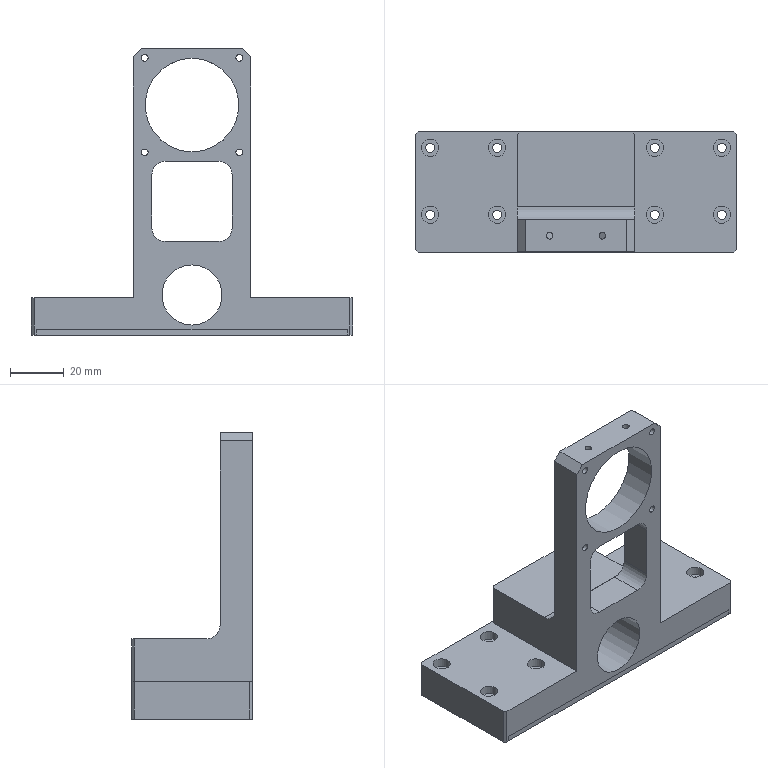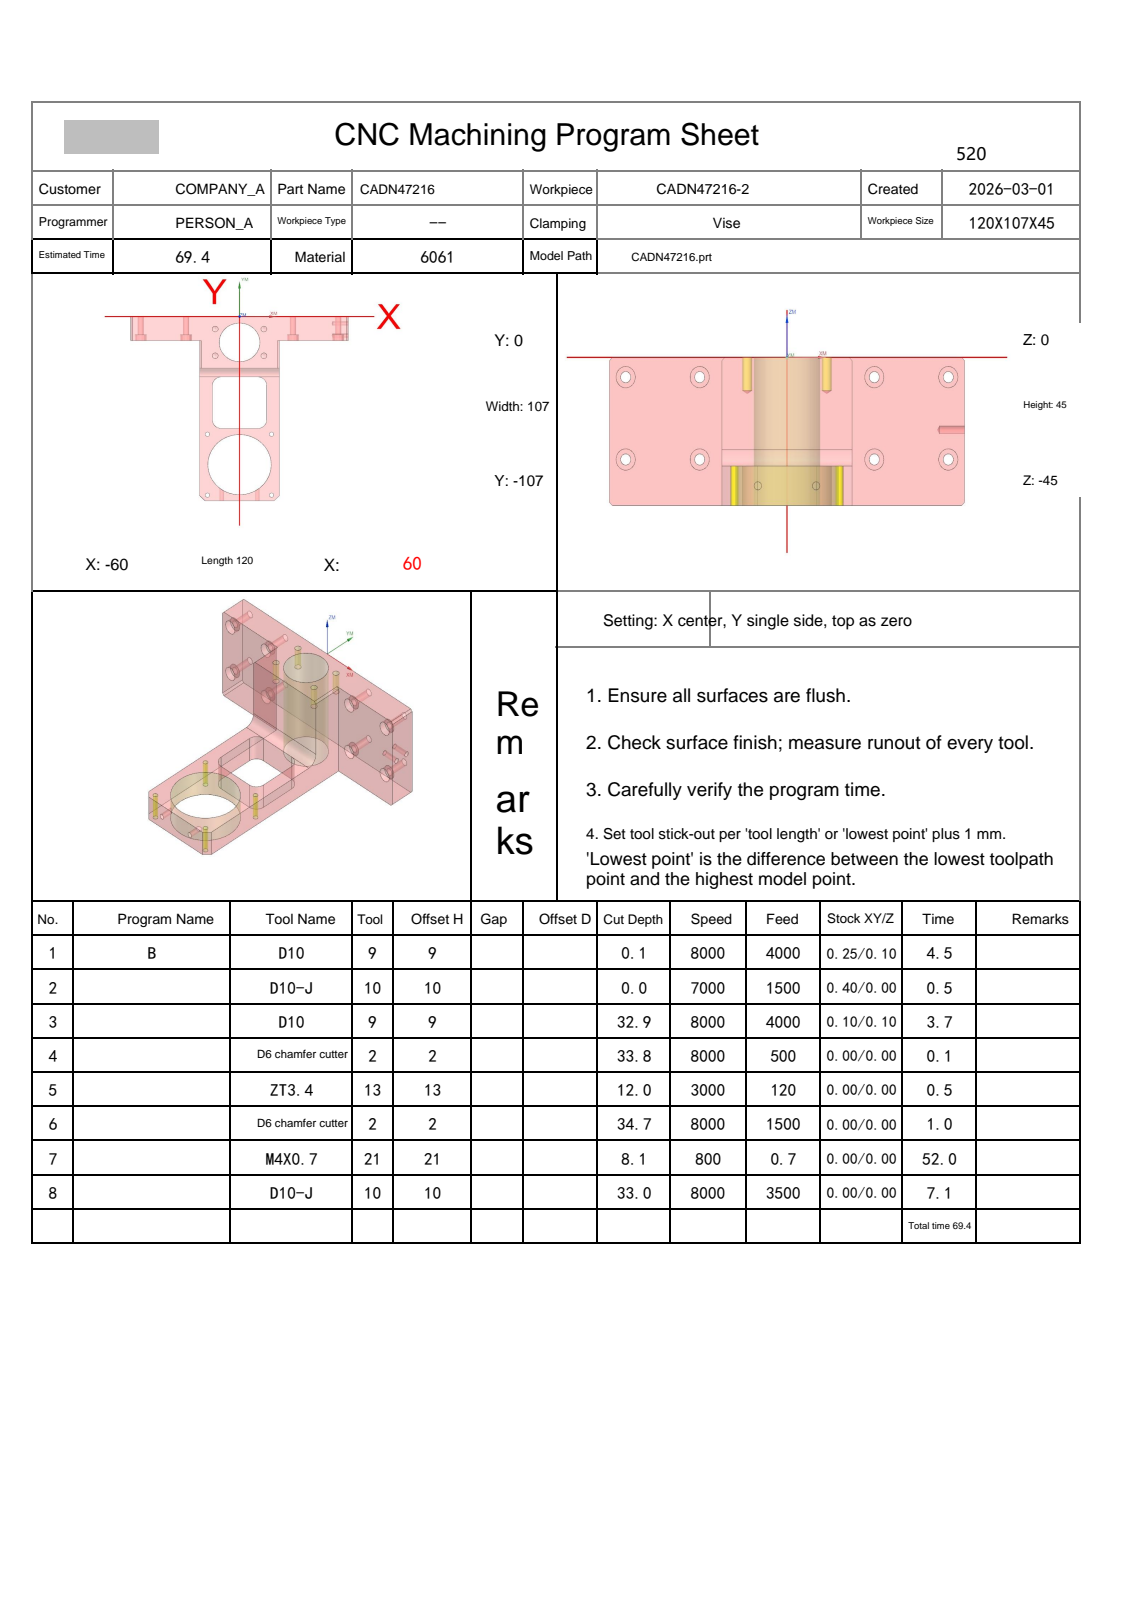NC program | NX | posted by the shop | part box 120 x 45 x 107 mm
Lines 1677 to 1756 of 8568:
N2 T10 M06
(D10-J  D=10. R=0. H=10 ce=0.40 di=0.00)
G00 G90 G54 X-2. Y7. M03 S7000
G43 H10 Z14.5
M08
Z1.5
G01 Z0.0 F1500.
Y3.
G03 X0.0 Y1. I2. J0.0
G01 X59.002
G02 X60. Y.002 I-.002 J-1.
G01 Y-14.002
G02 X59. Y-15. I-1. J.002
G01 X22.
Y-30.002
G02 X21.002 Y-31. I-1. J.002
G01 X-21.002
G02 X-22. Y-30.002 I.002 J1.
G01 Y-15.
X-59.002
G02 X-60. Y-14.002 I.002 J1.
G01 Y.002
G02 X-59.002 Y1. I1. J-.002
G01 X2.086
G02 X2.792 Y.708 I-.001 J-1.
G01 X7.207 Y-3.707
G03 X7.914 Y-4. I.707 J.707
G01 X54.003
G02 X55. Y-4.997 I-.003 J-1.
G01 Y-9.003
G02 X54.003 Y-10. I-1. J.003
G01 X22.
G03 X17. Y-15. I0.0 J-5.
G01 Y-25.003
G02 X16.003 Y-26. I-1. J.003
G01 X-16.003
G02 X-17. Y-25.003 I.003 J1.
G01 Y-15.
G03 X-22. Y-10. I-5. J0.0
G01 X-54.003
G02 X-55. Y-9.003 I.003 J1.
G01 Y-4.997
G02 X-54.003 Y-4. I1. J-.003
G01 X2.086
G02 X2.792 Y-4.292 I-.001 J-1.
G01 X7.207 Y-8.707
G03 X7.914 Y-9. I.707 J.707
G01 X12.205
G02 X13.202 Y-10. I-.003 J-1.
X13.094 Y-10.452 I-1. J0.0
G03 X12. Y-15. I8.906 J-4.548
G01 Y-20.003
G02 X11.003 Y-21. I-1. J.003
G01 X-11.003
G02 X-12. Y-20.003 I.003 J1.
G01 Y-15.
G03 X-13.094 Y-10.452 I-10. J0.0
G02 X-13.202 Y-10. I.892 J.452
X-12.205 Y-9. I1. J0.0
G01 X1.98
G02 X2.798 Y-9.426 I0.0 J-1.
G01 X5.766 Y-13.661
G03 X6.292 Y-14.044 I.819 J.574
G02 X7. Y-15. I-.292 J-.956
G01 Y-15.003
G02 X6.003 Y-16. I-1. J.003
G01 X-6.003
G02 X-7. Y-15. I.003 J1.
G01 Y-14.997
G02 X-6.003 Y-14. I1. J-.003
G01 X5.
X6.
G03 X8. Y-12. I0.0 J2.
G01 Z1.5
G00 Z14.5
G91 G28 Z0.0
M05
M09
G91 G28 Z0.0
M01